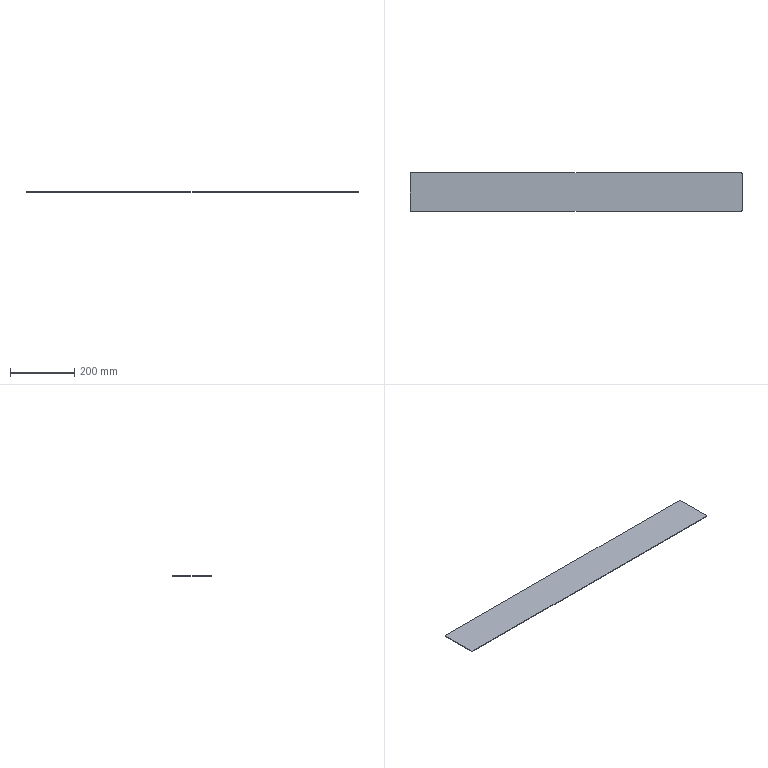Part | STEP file | KF-2212-070-002 | 1 solid | 10 faces | box 1036 x 120 x 2 mm | volume 248629 mm3 | plane 6 | cylinder 4 | commonest cylinder face diameters 5 x4
STEP:
#1=CARTESIAN_POINT('',(1026.,-7.5,0.));
#2=VERTEX_POINT('',#1);
#3=CARTESIAN_POINT('',(1026.,107.5,0.));
#4=VERTEX_POINT('',#3);
#5=CARTESIAN_POINT('',(1026.,-10.,0.));
#6=DIRECTION('',(0.,1.,0.));
#7=VECTOR('',#6,1000.);
#8=LINE('',#5,#7);
#9=EDGE_CURVE('',#2,#4,#8,.T.);
#10=ORIENTED_EDGE('',*,*,#9,.T.);
#11=CARTESIAN_POINT('',(1026.,107.5,2.));
#12=VERTEX_POINT('',#11);
#13=CARTESIAN_POINT('',(1026.,107.5,2.));
#14=DIRECTION('',(0.,0.,1.));
#15=VECTOR('',#14,1000.);
#16=LINE('',#13,#15);
#17=EDGE_CURVE('',#4,#12,#16,.T.);
#18=ORIENTED_EDGE('',*,*,#17,.T.);
#19=CARTESIAN_POINT('',(1026.,-7.5,2.));
#20=VERTEX_POINT('',#19);
#21=CARTESIAN_POINT('',(1026.,-10.,2.));
#22=DIRECTION('',(0.,1.,0.));
#23=VECTOR('',#22,1000.);
#24=LINE('',#21,#23);
#25=EDGE_CURVE('',#20,#12,#24,.T.);
#26=ORIENTED_EDGE('',*,*,#25,.F.);
#27=CARTESIAN_POINT('',(1026.,-7.5,2.));
#28=DIRECTION('',(0.,0.,-1.));
#29=VECTOR('',#28,1000.);
#30=LINE('',#27,#29);
#31=EDGE_CURVE('',#20,#2,#30,.T.);
#32=ORIENTED_EDGE('',*,*,#31,.T.);
#33=EDGE_LOOP('',(#10,#18,#26,#32));
#34=FACE_OUTER_BOUND('',#33,.T.);
#35=CARTESIAN_POINT('',(1026.,-10.,2.));
#36=DIRECTION('',(-1.,0.,0.));
#37=DIRECTION('',(0.,0.,1.));
#38=AXIS2_PLACEMENT_3D('',#35,#36,#37);
#39=PLANE('',#38);
#40=ADVANCED_FACE('',(#34),#39,.F.);
#41=CARTESIAN_POINT('',(1023.5,110.,2.));
#42=VERTEX_POINT('',#41);
#43=CARTESIAN_POINT('',(-7.5,110.,2.));
#44=VERTEX_POINT('',#43);
#45=CARTESIAN_POINT('',(1026.,110.,2.));
#46=DIRECTION('',(-1.,0.,0.));
#47=VECTOR('',#46,1000.);
#48=LINE('',#45,#47);
#49=EDGE_CURVE('',#42,#44,#48,.T.);
#50=ORIENTED_EDGE('',*,*,#49,.F.);
#51=CARTESIAN_POINT('',(1023.5,110.,0.));
#52=VERTEX_POINT('',#51);
#53=CARTESIAN_POINT('',(1023.5,110.,2.));
#54=DIRECTION('',(0.,0.,-1.));
#55=VECTOR('',#54,1000.);
#56=LINE('',#53,#55);
#57=EDGE_CURVE('',#42,#52,#56,.T.);
#58=ORIENTED_EDGE('',*,*,#57,.T.);
#59=CARTESIAN_POINT('',(-7.5,110.,0.));
#60=VERTEX_POINT('',#59);
#61=CARTESIAN_POINT('',(1026.,110.,0.));
#62=DIRECTION('',(-1.,0.,0.));
#63=VECTOR('',#62,1000.);
#64=LINE('',#61,#63);
#65=EDGE_CURVE('',#52,#60,#64,.T.);
#66=ORIENTED_EDGE('',*,*,#65,.T.);
#67=CARTESIAN_POINT('',(-7.5,110.,2.));
#68=DIRECTION('',(0.,0.,1.));
#69=VECTOR('',#68,1000.);
#70=LINE('',#67,#69);
#71=EDGE_CURVE('',#60,#44,#70,.T.);
#72=ORIENTED_EDGE('',*,*,#71,.T.);
#73=EDGE_LOOP('',(#50,#58,#66,#72));
#74=FACE_OUTER_BOUND('',#73,.T.);
#75=CARTESIAN_POINT('',(1026.,110.,2.));
#76=DIRECTION('',(0.,-1.,0.));
#77=DIRECTION('',(1.,0.,0.));
#78=AXIS2_PLACEMENT_3D('',#75,#76,#77);
#79=PLANE('',#78);
#80=ADVANCED_FACE('',(#74),#79,.F.);
#81=CARTESIAN_POINT('',(-10.,107.5,0.));
#82=VERTEX_POINT('',#81);
#83=CARTESIAN_POINT('',(-10.,-7.5,0.));
#84=VERTEX_POINT('',#83);
#85=CARTESIAN_POINT('',(-10.,-10.,0.));
#86=DIRECTION('',(0.,-1.,0.));
#87=VECTOR('',#86,1000.);
#88=LINE('',#85,#87);
#89=EDGE_CURVE('',#82,#84,#88,.T.);
#90=ORIENTED_EDGE('',*,*,#89,.T.);
#91=CARTESIAN_POINT('',(-10.,-7.5,2.));
#92=VERTEX_POINT('',#91);
#93=CARTESIAN_POINT('',(-10.,-7.5,2.));
#94=DIRECTION('',(0.,0.,1.));
#95=VECTOR('',#94,1000.);
#96=LINE('',#93,#95);
#97=EDGE_CURVE('',#84,#92,#96,.T.);
#98=ORIENTED_EDGE('',*,*,#97,.T.);
#99=CARTESIAN_POINT('',(-10.,107.5,2.));
#100=VERTEX_POINT('',#99);
#101=CARTESIAN_POINT('',(-10.,-10.,2.));
#102=DIRECTION('',(0.,-1.,0.));
#103=VECTOR('',#102,1000.);
#104=LINE('',#101,#103);
#105=EDGE_CURVE('',#100,#92,#104,.T.);
#106=ORIENTED_EDGE('',*,*,#105,.F.);
#107=CARTESIAN_POINT('',(-10.,107.5,2.));
#108=DIRECTION('',(0.,0.,-1.));
#109=VECTOR('',#108,1000.);
#110=LINE('',#107,#109);
#111=EDGE_CURVE('',#100,#82,#110,.T.);
#112=ORIENTED_EDGE('',*,*,#111,.T.);
#113=EDGE_LOOP('',(#90,#98,#106,#112));
#114=FACE_OUTER_BOUND('',#113,.T.);
#115=CARTESIAN_POINT('',(-10.,-10.,2.));
#116=DIRECTION('',(1.,0.,0.));
#117=DIRECTION('',(0.,0.,-1.));
#118=AXIS2_PLACEMENT_3D('',#115,#116,#117);
#119=PLANE('',#118);
#120=ADVANCED_FACE('',(#114),#119,.F.);
#121=CARTESIAN_POINT('',(-7.5,-10.,0.));
#122=VERTEX_POINT('',#121);
#123=CARTESIAN_POINT('',(1023.5,-10.,0.));
#124=VERTEX_POINT('',#123);
#125=CARTESIAN_POINT('',(1026.,-10.,0.));
#126=DIRECTION('',(1.,0.,0.));
#127=VECTOR('',#126,1000.);
#128=LINE('',#125,#127);
#129=EDGE_CURVE('',#122,#124,#128,.T.);
#130=ORIENTED_EDGE('',*,*,#129,.T.);
#131=CARTESIAN_POINT('',(1023.5,-10.,2.));
#132=VERTEX_POINT('',#131);
#133=CARTESIAN_POINT('',(1023.5,-10.,2.));
#134=DIRECTION('',(0.,0.,1.));
#135=VECTOR('',#134,1000.);
#136=LINE('',#133,#135);
#137=EDGE_CURVE('',#124,#132,#136,.T.);
#138=ORIENTED_EDGE('',*,*,#137,.T.);
#139=CARTESIAN_POINT('',(-7.5,-10.,2.));
#140=VERTEX_POINT('',#139);
#141=CARTESIAN_POINT('',(1026.,-10.,2.));
#142=DIRECTION('',(1.,0.,0.));
#143=VECTOR('',#142,1000.);
#144=LINE('',#141,#143);
#145=EDGE_CURVE('',#140,#132,#144,.T.);
#146=ORIENTED_EDGE('',*,*,#145,.F.);
#147=CARTESIAN_POINT('',(-7.5,-10.,2.));
#148=DIRECTION('',(0.,0.,-1.));
#149=VECTOR('',#148,1000.);
#150=LINE('',#147,#149);
#151=EDGE_CURVE('',#140,#122,#150,.T.);
#152=ORIENTED_EDGE('',*,*,#151,.T.);
#153=EDGE_LOOP('',(#130,#138,#146,#152));
#154=FACE_OUTER_BOUND('',#153,.T.);
#155=CARTESIAN_POINT('',(1026.,-10.,2.));
#156=DIRECTION('',(0.,1.,0.));
#157=DIRECTION('',(0.,0.,1.));
#158=AXIS2_PLACEMENT_3D('',#155,#156,#157);
#159=PLANE('',#158);
#160=ADVANCED_FACE('',(#154),#159,.F.);
#161=ORIENTED_EDGE('',*,*,#25,.T.);
#162=CARTESIAN_POINT('',(1023.5,107.5,2.));
#163=DIRECTION('',(0.,0.,1.));
#164=DIRECTION('',(1.,0.,0.));
#165=AXIS2_PLACEMENT_3D('',#162,#163,#164);
#166=CIRCLE('',#165,2.5);
#167=EDGE_CURVE('',#12,#42,#166,.T.);
#168=ORIENTED_EDGE('',*,*,#167,.T.);
#169=ORIENTED_EDGE('',*,*,#49,.T.);
#170=CARTESIAN_POINT('',(-7.5,107.5,2.));
#171=DIRECTION('',(0.,0.,1.));
#172=DIRECTION('',(1.,0.,0.));
#173=AXIS2_PLACEMENT_3D('',#170,#171,#172);
#174=CIRCLE('',#173,2.5);
#175=EDGE_CURVE('',#44,#100,#174,.T.);
#176=ORIENTED_EDGE('',*,*,#175,.T.);
#177=ORIENTED_EDGE('',*,*,#105,.T.);
#178=CARTESIAN_POINT('',(-7.5,-7.5,2.));
#179=DIRECTION('',(0.,0.,1.));
#180=DIRECTION('',(1.,0.,0.));
#181=AXIS2_PLACEMENT_3D('',#178,#179,#180);
#182=CIRCLE('',#181,2.5);
#183=EDGE_CURVE('',#92,#140,#182,.T.);
#184=ORIENTED_EDGE('',*,*,#183,.T.);
#185=ORIENTED_EDGE('',*,*,#145,.T.);
#186=CARTESIAN_POINT('',(1023.5,-7.5,2.));
#187=DIRECTION('',(0.,0.,1.));
#188=DIRECTION('',(1.,0.,0.));
#189=AXIS2_PLACEMENT_3D('',#186,#187,#188);
#190=CIRCLE('',#189,2.5);
#191=EDGE_CURVE('',#132,#20,#190,.T.);
#192=ORIENTED_EDGE('',*,*,#191,.T.);
#193=EDGE_LOOP('',(#161,#168,#169,#176,#177,#184,#185,#192));
#194=FACE_OUTER_BOUND('',#193,.T.);
#195=CARTESIAN_POINT('',(0.,0.,2.));
#196=DIRECTION('',(0.,0.,1.));
#197=DIRECTION('',(1.,0.,0.));
#198=AXIS2_PLACEMENT_3D('',#195,#196,#197);
#199=PLANE('',#198);
#200=ADVANCED_FACE('',(#194),#199,.T.);
#201=ORIENTED_EDGE('',*,*,#65,.F.);
#202=CARTESIAN_POINT('',(1023.5,107.5,0.));
#203=DIRECTION('',(0.,0.,-1.));
#204=DIRECTION('',(1.,0.,0.));
#205=AXIS2_PLACEMENT_3D('',#202,#203,#204);
#206=CIRCLE('',#205,2.5);
#207=EDGE_CURVE('',#52,#4,#206,.T.);
#208=ORIENTED_EDGE('',*,*,#207,.T.);
#209=ORIENTED_EDGE('',*,*,#9,.F.);
#210=CARTESIAN_POINT('',(1023.5,-7.5,0.));
#211=DIRECTION('',(0.,0.,-1.));
#212=DIRECTION('',(1.,0.,0.));
#213=AXIS2_PLACEMENT_3D('',#210,#211,#212);
#214=CIRCLE('',#213,2.5);
#215=EDGE_CURVE('',#2,#124,#214,.T.);
#216=ORIENTED_EDGE('',*,*,#215,.T.);
#217=ORIENTED_EDGE('',*,*,#129,.F.);
#218=CARTESIAN_POINT('',(-7.5,-7.5,0.));
#219=DIRECTION('',(0.,0.,-1.));
#220=DIRECTION('',(1.,0.,0.));
#221=AXIS2_PLACEMENT_3D('',#218,#219,#220);
#222=CIRCLE('',#221,2.5);
#223=EDGE_CURVE('',#122,#84,#222,.T.);
#224=ORIENTED_EDGE('',*,*,#223,.T.);
#225=ORIENTED_EDGE('',*,*,#89,.F.);
#226=CARTESIAN_POINT('',(-7.5,107.5,0.));
#227=DIRECTION('',(0.,0.,-1.));
#228=DIRECTION('',(1.,0.,0.));
#229=AXIS2_PLACEMENT_3D('',#226,#227,#228);
#230=CIRCLE('',#229,2.5);
#231=EDGE_CURVE('',#82,#60,#230,.T.);
#232=ORIENTED_EDGE('',*,*,#231,.T.);
#233=EDGE_LOOP('',(#201,#208,#209,#216,#217,#224,#225,#232));
#234=FACE_OUTER_BOUND('',#233,.T.);
#235=CARTESIAN_POINT('',(0.,0.,0.));
#236=DIRECTION('',(0.,0.,1.));
#237=DIRECTION('',(1.,0.,0.));
#238=AXIS2_PLACEMENT_3D('',#235,#236,#237);
#239=PLANE('',#238);
#240=ADVANCED_FACE('',(#234),#239,.F.);
#241=ORIENTED_EDGE('',*,*,#167,.F.);
#242=ORIENTED_EDGE('',*,*,#17,.F.);
#243=ORIENTED_EDGE('',*,*,#207,.F.);
#244=ORIENTED_EDGE('',*,*,#57,.F.);
#245=EDGE_LOOP('',(#241,#242,#243,#244));
#246=FACE_OUTER_BOUND('',#245,.T.);
#247=CARTESIAN_POINT('',(1023.5,107.5,2.));
#248=DIRECTION('',(0.,0.,-1.));
#249=DIRECTION('',(-1.,0.,0.));
#250=AXIS2_PLACEMENT_3D('',#247,#248,#249);
#251=CYLINDRICAL_SURFACE('',#250,2.5);
#252=ADVANCED_FACE('',(#246),#251,.T.);
#253=ORIENTED_EDGE('',*,*,#191,.F.);
#254=ORIENTED_EDGE('',*,*,#137,.F.);
#255=ORIENTED_EDGE('',*,*,#215,.F.);
#256=ORIENTED_EDGE('',*,*,#31,.F.);
#257=EDGE_LOOP('',(#253,#254,#255,#256));
#258=FACE_OUTER_BOUND('',#257,.T.);
#259=CARTESIAN_POINT('',(1023.5,-7.5,2.));
#260=DIRECTION('',(0.,0.,-1.));
#261=DIRECTION('',(-1.,0.,0.));
#262=AXIS2_PLACEMENT_3D('',#259,#260,#261);
#263=CYLINDRICAL_SURFACE('',#262,2.5);
#264=ADVANCED_FACE('',(#258),#263,.T.);
#265=ORIENTED_EDGE('',*,*,#183,.F.);
#266=ORIENTED_EDGE('',*,*,#97,.F.);
#267=ORIENTED_EDGE('',*,*,#223,.F.);
#268=ORIENTED_EDGE('',*,*,#151,.F.);
#269=EDGE_LOOP('',(#265,#266,#267,#268));
#270=FACE_OUTER_BOUND('',#269,.T.);
#271=CARTESIAN_POINT('',(-7.5,-7.5,2.));
#272=DIRECTION('',(0.,0.,-1.));
#273=DIRECTION('',(-1.,0.,0.));
#274=AXIS2_PLACEMENT_3D('',#271,#272,#273);
#275=CYLINDRICAL_SURFACE('',#274,2.5);
#276=ADVANCED_FACE('',(#270),#275,.T.);
#277=ORIENTED_EDGE('',*,*,#175,.F.);
#278=ORIENTED_EDGE('',*,*,#71,.F.);
#279=ORIENTED_EDGE('',*,*,#231,.F.);
#280=ORIENTED_EDGE('',*,*,#111,.F.);
#281=EDGE_LOOP('',(#277,#278,#279,#280));
#282=FACE_OUTER_BOUND('',#281,.T.);
#283=CARTESIAN_POINT('',(-7.5,107.5,2.));
#284=DIRECTION('',(0.,0.,-1.));
#285=DIRECTION('',(-1.,0.,0.));
#286=AXIS2_PLACEMENT_3D('',#283,#284,#285);
#287=CYLINDRICAL_SURFACE('',#286,2.5);
#288=ADVANCED_FACE('',(#282),#287,.T.);
#289=CLOSED_SHELL('',(#40,#80,#120,#160,#200,#240,#252,#264,#276,#288));
#290=MANIFOLD_SOLID_BREP('',#289);
#291=CARTESIAN_POINT('',(0.,0.,0.));
#292=DIRECTION('',(0.,0.,1.));
#293=DIRECTION('',(1.,0.,0.));
#294=AXIS2_PLACEMENT_3D('',#291,#292,#293);
#295=(LENGTH_UNIT()NAMED_UNIT(*)SI_UNIT(.MILLI.,.METRE.));
#296=UNCERTAINTY_MEASURE_WITH_UNIT(LENGTH_MEASURE(0.00001),#295,'','');
#297=(NAMED_UNIT(*)PLANE_ANGLE_UNIT()SI_UNIT($,.RADIAN.));
#298=(NAMED_UNIT(*)SI_UNIT($,.STERADIAN.)SOLID_ANGLE_UNIT());
#299=(GEOMETRIC_REPRESENTATION_CONTEXT(3)GLOBAL_UNCERTAINTY_ASSIGNED_CONTEXT((#296))GLOBAL_UNIT_ASSIGNED_CONTEXT((#295,#297,#298))REPRESENTATION_CONTEXT('',''));
#300=ADVANCED_BREP_SHAPE_REPRESENTATION('',(#290,#294),#299);